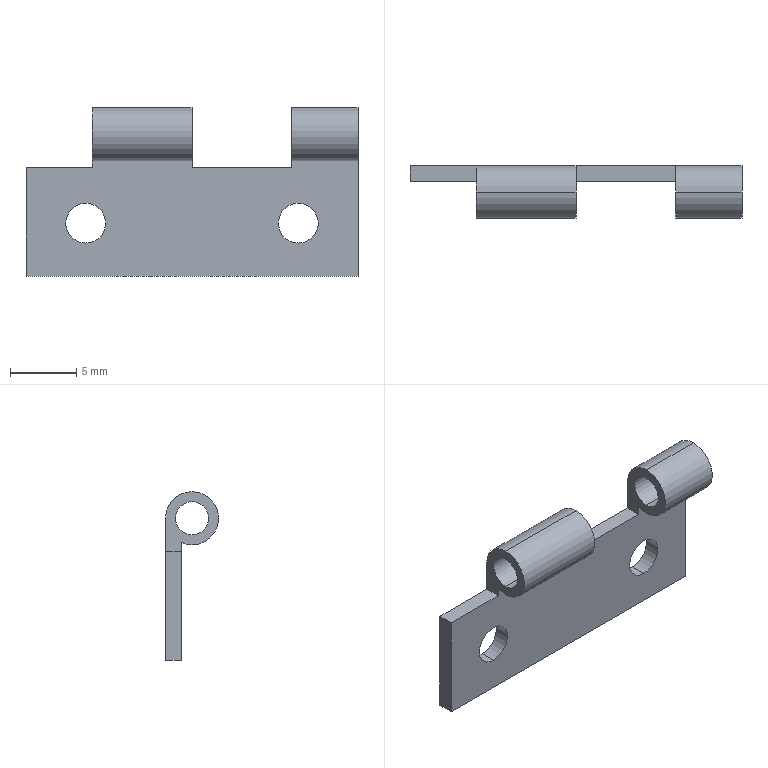Part | STEP file | 25 hinge-1 | 1 solid | 24 faces | box 25 x 4 x 12.7 mm | volume 342.439 mm3 | cylinder 14 | plane 10 | commonest cylinder face diameters 4 x6 2.5 x4 3 x4